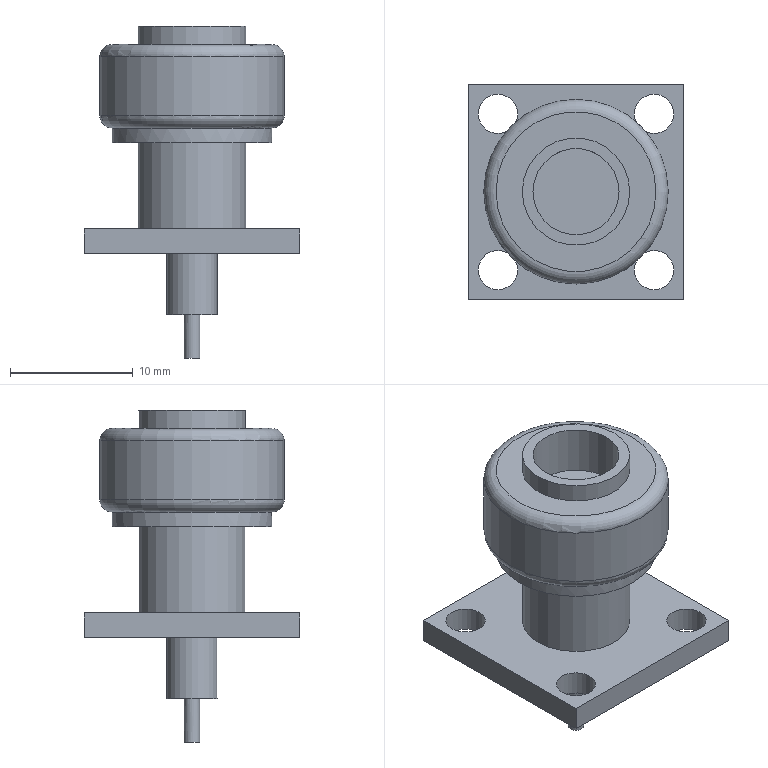Part | STEP file | N-KFD1005NT | 1 solid | 25 faces | box 17.5 x 17.5 x 27 mm | volume 2315 mm3 | plane 12 | cylinder 11 | torus 2 | commonest cylinder face diameters 3.2 x4 8.734 x2 1.27 x1 4.1 x1 7 x1 13 x1